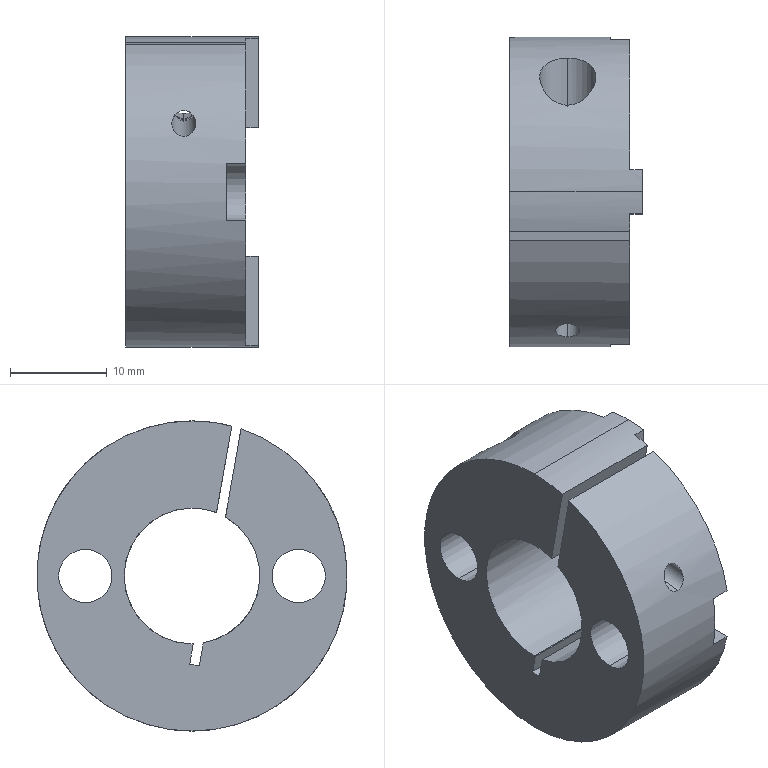Part | SolidWorks | features BaseBody 1 | 1 solid | 52 faces | box 13.7 x 32 x 32 mm | volume 6947 mm3 | cylinder 25 | plane 23 | cone 4 | commonest cylinder face diameters 2.459 x8 5.5 x4 14 x4 32 x3 3.8 x2 5.8 x2